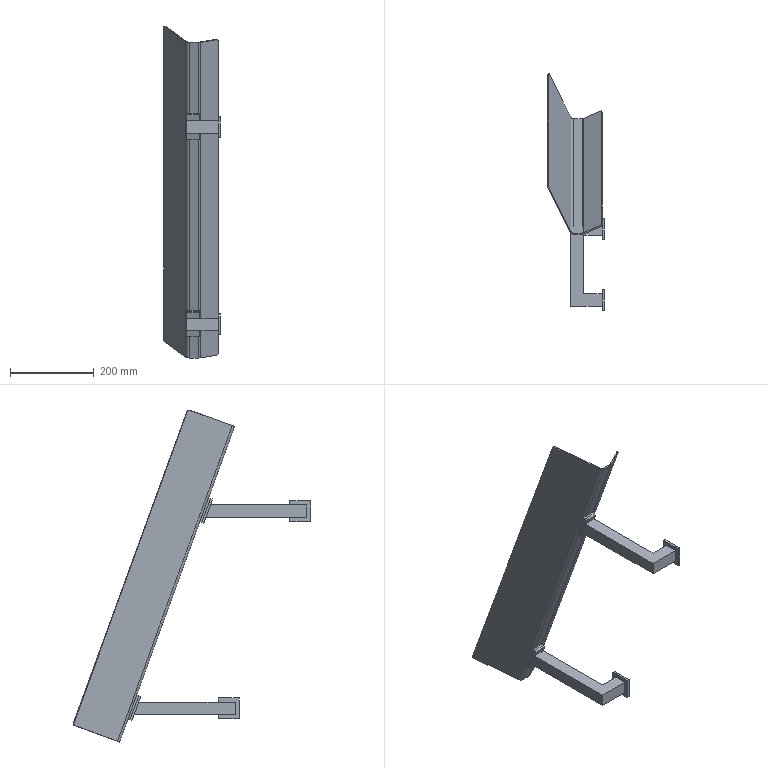Part | NX | features output director 8 | 7 solids | 68 faces | box 134.94 x 565.526 x 791.184 mm | volume 1060388 mm3 | plane 60 | cylinder 8 | commonest cylinder face diameters 10 x4 14 x2 20 x2